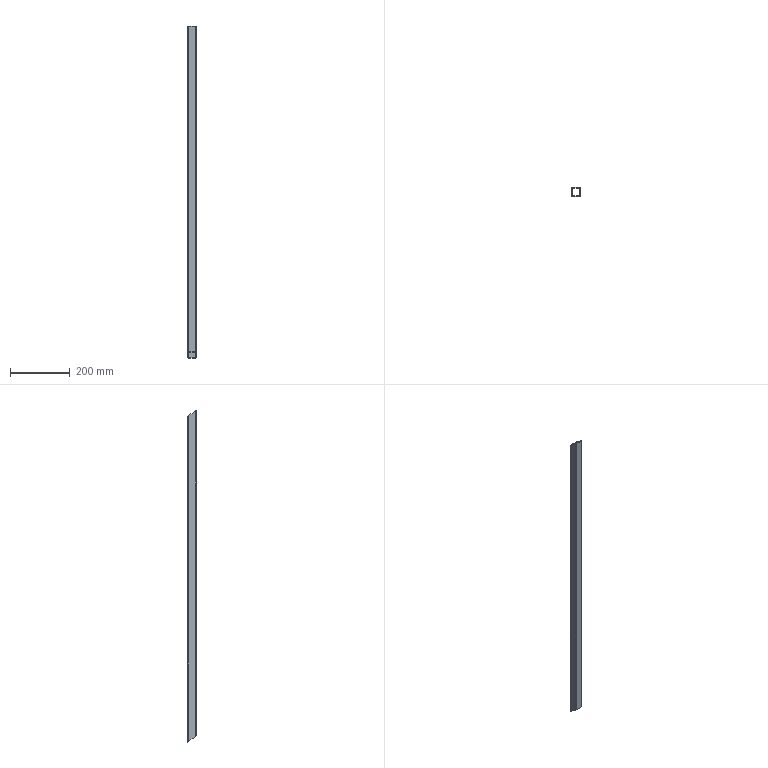Part | STEP file | CSN EN 10219-2 - 30 x 30 x 2  - 800 | 1 solid | 18 faces | box 30 x 30 x 1108 mm | volume 232357 mm3 | plane 10 | cylinder 8 | commonest cylinder face diameters 4 x4 8 x4